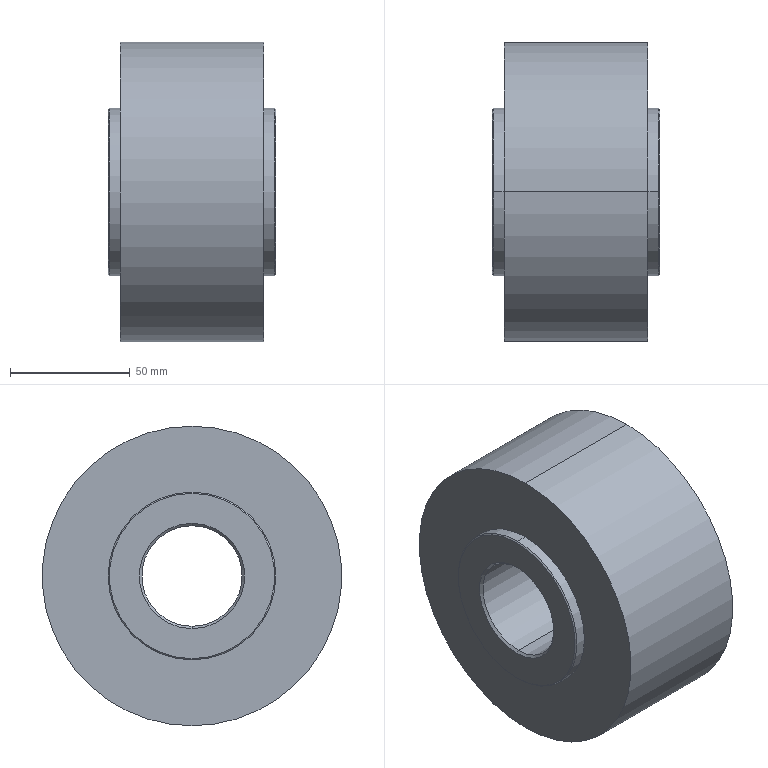Part | SolidWorks | features BaseBody 1 | 1 solid | 28 faces | box 70 x 125 x 125 mm | volume 635681 mm3 | cylinder 12 | cone 10 | plane 6 | commonest cylinder face diameters 70 x4 42 x2 52 x2 62 x2 125 x2
STEP:
#1=CARTESIAN_POINT('',(-30.,0.,-62.5));
#2=VERTEX_POINT('',#1);
#3=CARTESIAN_POINT('',(-30.,0.,62.5));
#4=VERTEX_POINT('',#3);
#5=CARTESIAN_POINT('',(-30.,0.,0.));
#6=DIRECTION('',(1.,0.,0.));
#7=DIRECTION('',(0.,0.,-1.));
#8=AXIS2_PLACEMENT_3D('',#5,#6,#7);
#9=CIRCLE('',#8,62.5);
#10=EDGE_CURVE('',#2,#4,#9,.T.);
#11=ORIENTED_EDGE('',*,*,#10,.T.);
#12=CARTESIAN_POINT('',(30.,0.,62.5));
#13=VERTEX_POINT('',#12);
#14=CARTESIAN_POINT('',(-38.5,0.,62.5));
#15=DIRECTION('',(1.,0.,0.));
#16=VECTOR('',#15,1000.);
#17=LINE('',#14,#16);
#18=EDGE_CURVE('',#4,#13,#17,.T.);
#19=ORIENTED_EDGE('',*,*,#18,.T.);
#20=CARTESIAN_POINT('',(30.,0.,-62.5));
#21=VERTEX_POINT('',#20);
#22=CARTESIAN_POINT('',(30.,0.,0.));
#23=DIRECTION('',(-1.,0.,0.));
#24=DIRECTION('',(0.,0.,-1.));
#25=AXIS2_PLACEMENT_3D('',#22,#23,#24);
#26=CIRCLE('',#25,62.5);
#27=EDGE_CURVE('',#13,#21,#26,.T.);
#28=ORIENTED_EDGE('',*,*,#27,.T.);
#29=CARTESIAN_POINT('',(-38.5,0.,-62.5));
#30=DIRECTION('',(1.,0.,0.));
#31=VECTOR('',#30,1000.);
#32=LINE('',#29,#31);
#33=EDGE_CURVE('',#2,#21,#32,.T.);
#34=ORIENTED_EDGE('',*,*,#33,.F.);
#35=EDGE_LOOP('',(#11,#19,#28,#34));
#36=FACE_OUTER_BOUND('',#35,.T.);
#37=CARTESIAN_POINT('',(-38.5,0.,0.));
#38=DIRECTION('',(1.,0.,0.));
#39=DIRECTION('',(0.,0.,-1.));
#40=AXIS2_PLACEMENT_3D('',#37,#38,#39);
#41=CYLINDRICAL_SURFACE('',#40,62.5);
#42=ADVANCED_FACE('',(#36),#41,.T.);
#43=CARTESIAN_POINT('',(30.,0.,35.));
#44=VERTEX_POINT('',#43);
#45=CARTESIAN_POINT('',(30.,0.,-35.));
#46=VERTEX_POINT('',#45);
#47=CARTESIAN_POINT('',(30.,0.,0.));
#48=DIRECTION('',(-1.,0.,0.));
#49=DIRECTION('',(0.,0.,-1.));
#50=AXIS2_PLACEMENT_3D('',#47,#48,#49);
#51=CIRCLE('',#50,35.);
#52=EDGE_CURVE('',#44,#46,#51,.T.);
#53=ORIENTED_EDGE('',*,*,#52,.F.);
#54=CARTESIAN_POINT('',(34.5,0.,35.));
#55=VERTEX_POINT('',#54);
#56=CARTESIAN_POINT('',(-38.5,0.,35.));
#57=DIRECTION('',(1.,0.,0.));
#58=VECTOR('',#57,1000.);
#59=LINE('',#56,#58);
#60=EDGE_CURVE('',#44,#55,#59,.T.);
#61=ORIENTED_EDGE('',*,*,#60,.T.);
#62=CARTESIAN_POINT('',(34.5,0.,-35.));
#63=VERTEX_POINT('',#62);
#64=CARTESIAN_POINT('',(34.5,0.,0.));
#65=DIRECTION('',(-1.,0.,0.));
#66=DIRECTION('',(0.,0.,-1.));
#67=AXIS2_PLACEMENT_3D('',#64,#65,#66);
#68=CIRCLE('',#67,35.);
#69=EDGE_CURVE('',#55,#63,#68,.T.);
#70=ORIENTED_EDGE('',*,*,#69,.T.);
#71=CARTESIAN_POINT('',(-38.5,0.,-35.));
#72=DIRECTION('',(1.,0.,0.));
#73=VECTOR('',#72,1000.);
#74=LINE('',#71,#73);
#75=EDGE_CURVE('',#46,#63,#74,.T.);
#76=ORIENTED_EDGE('',*,*,#75,.F.);
#77=EDGE_LOOP('',(#53,#61,#70,#76));
#78=FACE_OUTER_BOUND('',#77,.T.);
#79=CARTESIAN_POINT('',(-38.5,0.,0.));
#80=DIRECTION('',(1.,0.,0.));
#81=DIRECTION('',(0.,0.,-1.));
#82=AXIS2_PLACEMENT_3D('',#79,#80,#81);
#83=CYLINDRICAL_SURFACE('',#82,35.);
#84=ADVANCED_FACE('',(#78),#83,.T.);
#85=CARTESIAN_POINT('',(-34.5,0.,-35.));
#86=VERTEX_POINT('',#85);
#87=CARTESIAN_POINT('',(-34.5,0.,35.));
#88=VERTEX_POINT('',#87);
#89=CARTESIAN_POINT('',(-34.5,0.,0.));
#90=DIRECTION('',(1.,0.,0.));
#91=DIRECTION('',(0.,0.,-1.));
#92=AXIS2_PLACEMENT_3D('',#89,#90,#91);
#93=CIRCLE('',#92,35.);
#94=EDGE_CURVE('',#86,#88,#93,.T.);
#95=ORIENTED_EDGE('',*,*,#94,.T.);
#96=CARTESIAN_POINT('',(-30.,0.,35.));
#97=VERTEX_POINT('',#96);
#98=CARTESIAN_POINT('',(-38.5,0.,35.));
#99=DIRECTION('',(1.,0.,0.));
#100=VECTOR('',#99,1000.);
#101=LINE('',#98,#100);
#102=EDGE_CURVE('',#88,#97,#101,.T.);
#103=ORIENTED_EDGE('',*,*,#102,.T.);
#104=CARTESIAN_POINT('',(-30.,0.,-35.));
#105=VERTEX_POINT('',#104);
#106=CARTESIAN_POINT('',(-30.,0.,0.));
#107=DIRECTION('',(-1.,0.,0.));
#108=DIRECTION('',(0.,0.,-1.));
#109=AXIS2_PLACEMENT_3D('',#106,#107,#108);
#110=CIRCLE('',#109,35.);
#111=EDGE_CURVE('',#97,#105,#110,.T.);
#112=ORIENTED_EDGE('',*,*,#111,.T.);
#113=CARTESIAN_POINT('',(-38.5,0.,-35.));
#114=DIRECTION('',(1.,0.,0.));
#115=VECTOR('',#114,1000.);
#116=LINE('',#113,#115);
#117=EDGE_CURVE('',#86,#105,#116,.T.);
#118=ORIENTED_EDGE('',*,*,#117,.F.);
#119=EDGE_LOOP('',(#95,#103,#112,#118));
#120=FACE_OUTER_BOUND('',#119,.T.);
#121=CARTESIAN_POINT('',(-38.5,0.,0.));
#122=DIRECTION('',(1.,0.,0.));
#123=DIRECTION('',(0.,0.,-1.));
#124=AXIS2_PLACEMENT_3D('',#121,#122,#123);
#125=CYLINDRICAL_SURFACE('',#124,35.);
#126=ADVANCED_FACE('',(#120),#125,.T.);
#127=CARTESIAN_POINT('',(35.,0.,34.5));
#128=VERTEX_POINT('',#127);
#129=CARTESIAN_POINT('',(35.,0.,-34.5));
#130=VERTEX_POINT('',#129);
#131=CARTESIAN_POINT('',(35.,0.,0.));
#132=DIRECTION('',(-1.,0.,0.));
#133=DIRECTION('',(0.,0.,1.));
#134=AXIS2_PLACEMENT_3D('',#131,#132,#133);
#135=CIRCLE('',#134,34.5);
#136=EDGE_CURVE('',#128,#130,#135,.T.);
#137=ORIENTED_EDGE('',*,*,#136,.T.);
#138=CARTESIAN_POINT('',(34.5,0.,-35.));
#139=DIRECTION('',(-0.7071,0.,-0.7071));
#140=VECTOR('',#139,1000.);
#141=LINE('',#138,#140);
#142=EDGE_CURVE('',#130,#63,#141,.T.);
#143=ORIENTED_EDGE('',*,*,#142,.T.);
#144=ORIENTED_EDGE('',*,*,#69,.F.);
#145=CARTESIAN_POINT('',(34.5,0.,35.));
#146=DIRECTION('',(-0.7071,0.,0.7071));
#147=VECTOR('',#146,1000.);
#148=LINE('',#145,#147);
#149=EDGE_CURVE('',#128,#55,#148,.T.);
#150=ORIENTED_EDGE('',*,*,#149,.F.);
#151=EDGE_LOOP('',(#137,#143,#144,#150));
#152=FACE_OUTER_BOUND('',#151,.T.);
#153=CARTESIAN_POINT('',(34.5,0.,0.));
#154=DIRECTION('',(-1.,0.,0.));
#155=DIRECTION('',(0.,0.,1.));
#156=AXIS2_PLACEMENT_3D('',#153,#154,#155);
#157=CONICAL_SURFACE('',#156,35.,0.7854);
#158=ADVANCED_FACE('',(#152),#157,.T.);
#159=CARTESIAN_POINT('',(-35.,0.,-34.5));
#160=VERTEX_POINT('',#159);
#161=CARTESIAN_POINT('',(-35.,0.,34.5));
#162=VERTEX_POINT('',#161);
#163=CARTESIAN_POINT('',(-35.,0.,0.));
#164=DIRECTION('',(1.,0.,0.));
#165=DIRECTION('',(0.,0.,-1.));
#166=AXIS2_PLACEMENT_3D('',#163,#164,#165);
#167=CIRCLE('',#166,34.5);
#168=EDGE_CURVE('',#160,#162,#167,.T.);
#169=ORIENTED_EDGE('',*,*,#168,.T.);
#170=CARTESIAN_POINT('',(-34.5,0.,35.));
#171=DIRECTION('',(0.7071,0.,0.7071));
#172=VECTOR('',#171,1000.);
#173=LINE('',#170,#172);
#174=EDGE_CURVE('',#162,#88,#173,.T.);
#175=ORIENTED_EDGE('',*,*,#174,.T.);
#176=ORIENTED_EDGE('',*,*,#94,.F.);
#177=CARTESIAN_POINT('',(-34.5,0.,-35.));
#178=DIRECTION('',(0.7071,0.,-0.7071));
#179=VECTOR('',#178,1000.);
#180=LINE('',#177,#179);
#181=EDGE_CURVE('',#160,#86,#180,.T.);
#182=ORIENTED_EDGE('',*,*,#181,.F.);
#183=EDGE_LOOP('',(#169,#175,#176,#182));
#184=FACE_OUTER_BOUND('',#183,.T.);
#185=CARTESIAN_POINT('',(-34.5,0.,0.));
#186=DIRECTION('',(1.,0.,0.));
#187=DIRECTION('',(0.,0.,-1.));
#188=AXIS2_PLACEMENT_3D('',#185,#186,#187);
#189=CONICAL_SURFACE('',#188,35.,0.7854);
#190=ADVANCED_FACE('',(#184),#189,.T.);
#191=CARTESIAN_POINT('',(34.,0.,31.));
#192=VERTEX_POINT('',#191);
#193=CARTESIAN_POINT('',(34.,0.,-31.));
#194=VERTEX_POINT('',#193);
#195=CARTESIAN_POINT('',(34.,0.,0.));
#196=DIRECTION('',(1.,0.,0.));
#197=DIRECTION('',(0.,0.,-1.));
#198=AXIS2_PLACEMENT_3D('',#195,#196,#197);
#199=CIRCLE('',#198,31.);
#200=EDGE_CURVE('',#192,#194,#199,.T.);
#201=ORIENTED_EDGE('',*,*,#200,.F.);
#202=CARTESIAN_POINT('',(35.,0.,32.));
#203=VERTEX_POINT('',#202);
#204=CARTESIAN_POINT('',(35.,0.,32.));
#205=DIRECTION('',(0.7071,0.,0.7071));
#206=VECTOR('',#205,1000.);
#207=LINE('',#204,#206);
#208=EDGE_CURVE('',#192,#203,#207,.T.);
#209=ORIENTED_EDGE('',*,*,#208,.T.);
#210=CARTESIAN_POINT('',(35.,0.,-32.));
#211=VERTEX_POINT('',#210);
#212=CARTESIAN_POINT('',(35.,0.,0.));
#213=DIRECTION('',(-1.,0.,0.));
#214=DIRECTION('',(0.,0.,-1.));
#215=AXIS2_PLACEMENT_3D('',#212,#213,#214);
#216=CIRCLE('',#215,32.);
#217=EDGE_CURVE('',#211,#203,#216,.T.);
#218=ORIENTED_EDGE('',*,*,#217,.F.);
#219=CARTESIAN_POINT('',(35.,0.,-32.));
#220=DIRECTION('',(0.7071,0.,-0.7071));
#221=VECTOR('',#220,1000.);
#222=LINE('',#219,#221);
#223=EDGE_CURVE('',#194,#211,#222,.T.);
#224=ORIENTED_EDGE('',*,*,#223,.F.);
#225=EDGE_LOOP('',(#201,#209,#218,#224));
#226=FACE_OUTER_BOUND('',#225,.T.);
#227=CARTESIAN_POINT('',(35.,0.,0.));
#228=DIRECTION('',(1.,0.,0.));
#229=DIRECTION('',(0.,0.,-1.));
#230=AXIS2_PLACEMENT_3D('',#227,#228,#229);
#231=CONICAL_SURFACE('',#230,32.,0.7854);
#232=ADVANCED_FACE('',(#226),#231,.F.);
#233=CARTESIAN_POINT('',(-34.,0.,-21.));
#234=VERTEX_POINT('',#233);
#235=CARTESIAN_POINT('',(-34.,0.,21.));
#236=VERTEX_POINT('',#235);
#237=CARTESIAN_POINT('',(-34.,0.,0.));
#238=DIRECTION('',(-1.,0.,0.));
#239=DIRECTION('',(0.,0.,-1.));
#240=AXIS2_PLACEMENT_3D('',#237,#238,#239);
#241=CIRCLE('',#240,21.);
#242=EDGE_CURVE('',#234,#236,#241,.T.);
#243=ORIENTED_EDGE('',*,*,#242,.F.);
#244=CARTESIAN_POINT('',(-35.,0.,-22.));
#245=VERTEX_POINT('',#244);
#246=CARTESIAN_POINT('',(-35.,0.,-22.));
#247=DIRECTION('',(-0.7071,0.,-0.7071));
#248=VECTOR('',#247,1000.);
#249=LINE('',#246,#248);
#250=EDGE_CURVE('',#234,#245,#249,.T.);
#251=ORIENTED_EDGE('',*,*,#250,.T.);
#252=CARTESIAN_POINT('',(-35.,0.,22.));
#253=VERTEX_POINT('',#252);
#254=CARTESIAN_POINT('',(-35.,0.,0.));
#255=DIRECTION('',(-1.,0.,0.));
#256=DIRECTION('',(0.,0.,1.));
#257=AXIS2_PLACEMENT_3D('',#254,#255,#256);
#258=CIRCLE('',#257,22.);
#259=EDGE_CURVE('',#245,#253,#258,.T.);
#260=ORIENTED_EDGE('',*,*,#259,.T.);
#261=CARTESIAN_POINT('',(-35.,0.,22.));
#262=DIRECTION('',(-0.7071,0.,0.7071));
#263=VECTOR('',#262,1000.);
#264=LINE('',#261,#263);
#265=EDGE_CURVE('',#236,#253,#264,.T.);
#266=ORIENTED_EDGE('',*,*,#265,.F.);
#267=EDGE_LOOP('',(#243,#251,#260,#266));
#268=FACE_OUTER_BOUND('',#267,.T.);
#269=CARTESIAN_POINT('',(-35.,0.,0.));
#270=DIRECTION('',(-1.,0.,0.));
#271=DIRECTION('',(0.,0.,1.));
#272=AXIS2_PLACEMENT_3D('',#269,#270,#271);
#273=CONICAL_SURFACE('',#272,22.,0.7854);
#274=ADVANCED_FACE('',(#268),#273,.F.);
#275=CARTESIAN_POINT('',(13.,0.,31.));
#276=VERTEX_POINT('',#275);
#277=CARTESIAN_POINT('',(13.,0.,-31.));
#278=VERTEX_POINT('',#277);
#279=CARTESIAN_POINT('',(13.,0.,0.));
#280=DIRECTION('',(1.,0.,0.));
#281=DIRECTION('',(0.,0.,-1.));
#282=AXIS2_PLACEMENT_3D('',#279,#280,#281);
#283=CIRCLE('',#282,31.);
#284=EDGE_CURVE('',#276,#278,#283,.T.);
#285=ORIENTED_EDGE('',*,*,#284,.F.);
#286=CARTESIAN_POINT('',(-38.5,0.,31.));
#287=DIRECTION('',(1.,0.,0.));
#288=VECTOR('',#287,1000.);
#289=LINE('',#286,#288);
#290=EDGE_CURVE('',#276,#192,#289,.T.);
#291=ORIENTED_EDGE('',*,*,#290,.T.);
#292=ORIENTED_EDGE('',*,*,#200,.T.);
#293=CARTESIAN_POINT('',(-38.5,0.,-31.));
#294=DIRECTION('',(1.,0.,0.));
#295=VECTOR('',#294,1000.);
#296=LINE('',#293,#295);
#297=EDGE_CURVE('',#278,#194,#296,.T.);
#298=ORIENTED_EDGE('',*,*,#297,.F.);
#299=EDGE_LOOP('',(#285,#291,#292,#298));
#300=FACE_OUTER_BOUND('',#299,.T.);
#301=CARTESIAN_POINT('',(-38.5,0.,0.));
#302=DIRECTION('',(1.,0.,0.));
#303=DIRECTION('',(0.,0.,-1.));
#304=AXIS2_PLACEMENT_3D('',#301,#302,#303);
#305=CYLINDRICAL_SURFACE('',#304,31.);
#306=ADVANCED_FACE('',(#300),#305,.F.);
#307=ORIENTED_EDGE('',*,*,#242,.T.);
#308=CARTESIAN_POINT('',(4.,0.,21.));
#309=VERTEX_POINT('',#308);
#310=CARTESIAN_POINT('',(-38.5,0.,21.));
#311=DIRECTION('',(1.,0.,0.));
#312=VECTOR('',#311,1000.);
#313=LINE('',#310,#312);
#314=EDGE_CURVE('',#236,#309,#313,.T.);
#315=ORIENTED_EDGE('',*,*,#314,.T.);
#316=CARTESIAN_POINT('',(4.,0.,-21.));
#317=VERTEX_POINT('',#316);
#318=CARTESIAN_POINT('',(4.,0.,0.));
#319=DIRECTION('',(-1.,0.,0.));
#320=DIRECTION('',(0.,0.,-1.));
#321=AXIS2_PLACEMENT_3D('',#318,#319,#320);
#322=CIRCLE('',#321,21.);
#323=EDGE_CURVE('',#317,#309,#322,.T.);
#324=ORIENTED_EDGE('',*,*,#323,.F.);
#325=CARTESIAN_POINT('',(-38.5,0.,-21.));
#326=DIRECTION('',(1.,0.,0.));
#327=VECTOR('',#326,1000.);
#328=LINE('',#325,#327);
#329=EDGE_CURVE('',#234,#317,#328,.T.);
#330=ORIENTED_EDGE('',*,*,#329,.F.);
#331=EDGE_LOOP('',(#307,#315,#324,#330));
#332=FACE_OUTER_BOUND('',#331,.T.);
#333=CARTESIAN_POINT('',(-38.5,0.,0.));
#334=DIRECTION('',(1.,0.,0.));
#335=DIRECTION('',(0.,0.,-1.));
#336=AXIS2_PLACEMENT_3D('',#333,#334,#335);
#337=CYLINDRICAL_SURFACE('',#336,21.);
#338=ADVANCED_FACE('',(#332),#337,.F.);
#339=ORIENTED_EDGE('',*,*,#323,.T.);
#340=CARTESIAN_POINT('',(5.,0.,22.));
#341=VERTEX_POINT('',#340);
#342=CARTESIAN_POINT('',(5.,0.,22.));
#343=DIRECTION('',(0.7071,0.,0.7071));
#344=VECTOR('',#343,1000.);
#345=LINE('',#342,#344);
#346=EDGE_CURVE('',#309,#341,#345,.T.);
#347=ORIENTED_EDGE('',*,*,#346,.T.);
#348=CARTESIAN_POINT('',(5.,0.,-22.));
#349=VERTEX_POINT('',#348);
#350=CARTESIAN_POINT('',(5.,0.,0.));
#351=DIRECTION('',(-1.,0.,0.));
#352=DIRECTION('',(0.,0.,-1.));
#353=AXIS2_PLACEMENT_3D('',#350,#351,#352);
#354=CIRCLE('',#353,22.);
#355=EDGE_CURVE('',#349,#341,#354,.T.);
#356=ORIENTED_EDGE('',*,*,#355,.F.);
#357=CARTESIAN_POINT('',(5.,0.,-22.));
#358=DIRECTION('',(0.7071,0.,-0.7071));
#359=VECTOR('',#358,1000.);
#360=LINE('',#357,#359);
#361=EDGE_CURVE('',#317,#349,#360,.T.);
#362=ORIENTED_EDGE('',*,*,#361,.F.);
#363=EDGE_LOOP('',(#339,#347,#356,#362));
#364=FACE_OUTER_BOUND('',#363,.T.);
#365=CARTESIAN_POINT('',(5.,0.,0.));
#366=DIRECTION('',(1.,0.,0.));
#367=DIRECTION('',(0.,0.,-1.));
#368=AXIS2_PLACEMENT_3D('',#365,#366,#367);
#369=CONICAL_SURFACE('',#368,22.,0.7854);
#370=ADVANCED_FACE('',(#364),#369,.F.);
#371=CARTESIAN_POINT('',(5.,0.,26.));
#372=VERTEX_POINT('',#371);
#373=CARTESIAN_POINT('',(5.,0.,-26.));
#374=VERTEX_POINT('',#373);
#375=CARTESIAN_POINT('',(5.,0.,0.));
#376=DIRECTION('',(1.,0.,0.));
#377=DIRECTION('',(0.,0.,-1.));
#378=AXIS2_PLACEMENT_3D('',#375,#376,#377);
#379=CIRCLE('',#378,26.);
#380=EDGE_CURVE('',#372,#374,#379,.T.);
#381=ORIENTED_EDGE('',*,*,#380,.F.);
#382=CARTESIAN_POINT('',(13.,0.,26.));
#383=VERTEX_POINT('',#382);
#384=CARTESIAN_POINT('',(-38.5,0.,26.));
#385=DIRECTION('',(1.,0.,0.));
#386=VECTOR('',#385,1000.);
#387=LINE('',#384,#386);
#388=EDGE_CURVE('',#372,#383,#387,.T.);
#389=ORIENTED_EDGE('',*,*,#388,.T.);
#390=CARTESIAN_POINT('',(13.,0.,-26.));
#391=VERTEX_POINT('',#390);
#392=CARTESIAN_POINT('',(13.,0.,0.));
#393=DIRECTION('',(-1.,0.,0.));
#394=DIRECTION('',(0.,0.,-1.));
#395=AXIS2_PLACEMENT_3D('',#392,#393,#394);
#396=CIRCLE('',#395,26.);
#397=EDGE_CURVE('',#391,#383,#396,.T.);
#398=ORIENTED_EDGE('',*,*,#397,.F.);
#399=CARTESIAN_POINT('',(-38.5,0.,-26.));
#400=DIRECTION('',(1.,0.,0.));
#401=VECTOR('',#400,1000.);
#402=LINE('',#399,#401);
#403=EDGE_CURVE('',#374,#391,#402,.T.);
#404=ORIENTED_EDGE('',*,*,#403,.F.);
#405=EDGE_LOOP('',(#381,#389,#398,#404));
#406=FACE_OUTER_BOUND('',#405,.T.);
#407=CARTESIAN_POINT('',(-38.5,0.,0.));
#408=DIRECTION('',(1.,0.,0.));
#409=DIRECTION('',(0.,0.,-1.));
#410=AXIS2_PLACEMENT_3D('',#407,#408,#409);
#411=CYLINDRICAL_SURFACE('',#410,26.);
#412=ADVANCED_FACE('',(#406),#411,.F.);
#413=ORIENTED_EDGE('',*,*,#18,.F.);
#414=CARTESIAN_POINT('',(-30.,0.,0.));
#415=DIRECTION('',(1.,0.,0.));
#416=DIRECTION('',(0.,0.,-1.));
#417=AXIS2_PLACEMENT_3D('',#414,#415,#416);
#418=CIRCLE('',#417,62.5);
#419=EDGE_CURVE('',#4,#2,#418,.T.);
#420=ORIENTED_EDGE('',*,*,#419,.T.);
#421=ORIENTED_EDGE('',*,*,#33,.T.);
#422=CARTESIAN_POINT('',(30.,0.,0.));
#423=DIRECTION('',(-1.,0.,0.));
#424=DIRECTION('',(0.,0.,-1.));
#425=AXIS2_PLACEMENT_3D('',#422,#423,#424);
#426=CIRCLE('',#425,62.5);
#427=EDGE_CURVE('',#21,#13,#426,.T.);
#428=ORIENTED_EDGE('',*,*,#427,.T.);
#429=EDGE_LOOP('',(#413,#420,#421,#428));
#430=FACE_OUTER_BOUND('',#429,.T.);
#431=CARTESIAN_POINT('',(-38.5,0.,0.));
#432=DIRECTION('',(1.,0.,0.));
#433=DIRECTION('',(0.,0.,-1.));
#434=AXIS2_PLACEMENT_3D('',#431,#432,#433);
#435=CYLINDRICAL_SURFACE('',#434,62.5);
#436=ADVANCED_FACE('',(#430),#435,.T.);
#437=CARTESIAN_POINT('',(30.,0.,0.));
#438=DIRECTION('',(-1.,0.,0.));
#439=DIRECTION('',(0.,0.,-1.));
#440=AXIS2_PLACEMENT_3D('',#437,#438,#439);
#441=CIRCLE('',#440,35.);
#442=EDGE_CURVE('',#46,#44,#441,.T.);
#443=ORIENTED_EDGE('',*,*,#442,.T.);
#444=ORIENTED_EDGE('',*,*,#52,.T.);
#445=EDGE_LOOP('',(#443,#444));
#446=FACE_BOUND('',#445,.T.);
#447=ORIENTED_EDGE('',*,*,#427,.F.);
#448=ORIENTED_EDGE('',*,*,#27,.F.);
#449=EDGE_LOOP('',(#447,#448));
#450=FACE_OUTER_BOUND('',#449,.T.);
#451=CARTESIAN_POINT('',(30.,0.,0.));
#452=DIRECTION('',(1.,0.,0.));
#453=DIRECTION('',(0.,0.,-1.));
#454=AXIS2_PLACEMENT_3D('',#451,#452,#453);
#455=PLANE('',#454);
#456=ADVANCED_FACE('',(#446,#450),#455,.T.);
#457=CARTESIAN_POINT('',(-30.,0.,0.));
#458=DIRECTION('',(-1.,0.,0.));
#459=DIRECTION('',(0.,0.,-1.));
#460=AXIS2_PLACEMENT_3D('',#457,#458,#459);
#461=CIRCLE('',#460,35.);
#462=EDGE_CURVE('',#105,#97,#461,.T.);
#463=ORIENTED_EDGE('',*,*,#462,.F.);
#464=ORIENTED_EDGE('',*,*,#111,.F.);
#465=EDGE_LOOP('',(#463,#464));
#466=FACE_BOUND('',#465,.T.);
#467=ORIENTED_EDGE('',*,*,#10,.F.);
#468=ORIENTED_EDGE('',*,*,#419,.F.);
#469=EDGE_LOOP('',(#467,#468));
#470=FACE_OUTER_BOUND('',#469,.T.);
#471=CARTESIAN_POINT('',(-30.,0.,0.));
#472=DIRECTION('',(1.,0.,0.));
#473=DIRECTION('',(0.,0.,-1.));
#474=AXIS2_PLACEMENT_3D('',#471,#472,#473);
#475=PLANE('',#474);
#476=ADVANCED_FACE('',(#466,#470),#475,.F.);
#477=ORIENTED_EDGE('',*,*,#60,.F.);
#478=ORIENTED_EDGE('',*,*,#442,.F.);
#479=ORIENTED_EDGE('',*,*,#75,.T.);
#480=CARTESIAN_POINT('',(34.5,0.,0.));
#481=DIRECTION('',(-1.,0.,0.));
#482=DIRECTION('',(0.,0.,-1.));
#483=AXIS2_PLACEMENT_3D('',#480,#481,#482);
#484=CIRCLE('',#483,35.);
#485=EDGE_CURVE('',#63,#55,#484,.T.);
#486=ORIENTED_EDGE('',*,*,#485,.T.);
#487=EDGE_LOOP('',(#477,#478,#479,#486));
#488=FACE_OUTER_BOUND('',#487,.T.);
#489=CARTESIAN_POINT('',(-38.5,0.,0.));
#490=DIRECTION('',(1.,0.,0.));
#491=DIRECTION('',(0.,0.,-1.));
#492=AXIS2_PLACEMENT_3D('',#489,#490,#491);
#493=CYLINDRICAL_SURFACE('',#492,35.);
#494=ADVANCED_FACE('',(#488),#493,.T.);
#495=ORIENTED_EDGE('',*,*,#102,.F.);
#496=CARTESIAN_POINT('',(-34.5,0.,0.));
#497=DIRECTION('',(1.,0.,0.));
#498=DIRECTION('',(0.,0.,-1.));
#499=AXIS2_PLACEMENT_3D('',#496,#497,#498);
#500=CIRCLE('',#499,35.);
#501=EDGE_CURVE('',#88,#86,#500,.T.);
#502=ORIENTED_EDGE('',*,*,#501,.T.);
#503=ORIENTED_EDGE('',*,*,#117,.T.);
#504=ORIENTED_EDGE('',*,*,#462,.T.);
#505=EDGE_LOOP('',(#495,#502,#503,#504));
#506=FACE_OUTER_BOUND('',#505,.T.);
#507=CARTESIAN_POINT('',(-38.5,0.,0.));
#508=DIRECTION('',(1.,0.,0.));
#509=DIRECTION('',(0.,0.,-1.));
#510=AXIS2_PLACEMENT_3D('',#507,#508,#509);
#511=CYLINDRICAL_SURFACE('',#510,35.);
#512=ADVANCED_FACE('',(#506),#511,.T.);
#513=ORIENTED_EDGE('',*,*,#142,.F.);
#514=CARTESIAN_POINT('',(35.,0.,0.));
#515=DIRECTION('',(-1.,0.,0.));
#516=DIRECTION('',(0.,0.,1.));
#517=AXIS2_PLACEMENT_3D('',#514,#515,#516);
#518=CIRCLE('',#517,34.5);
#519=EDGE_CURVE('',#130,#128,#518,.T.);
#520=ORIENTED_EDGE('',*,*,#519,.T.);
#521=ORIENTED_EDGE('',*,*,#149,.T.);
#522=ORIENTED_EDGE('',*,*,#485,.F.);
#523=EDGE_LOOP('',(#513,#520,#521,#522));
#524=FACE_OUTER_BOUND('',#523,.T.);
#525=CARTESIAN_POINT('',(34.5,0.,0.));
#526=DIRECTION('',(-1.,0.,0.));
#527=DIRECTION('',(0.,0.,1.));
#528=AXIS2_PLACEMENT_3D('',#525,#526,#527);
#529=CONICAL_SURFACE('',#528,35.,0.7854);
#530=ADVANCED_FACE('',(#524),#529,.T.);
#531=ORIENTED_EDGE('',*,*,#174,.F.);
#532=CARTESIAN_POINT('',(-35.,0.,0.));
#533=DIRECTION('',(1.,0.,0.));
#534=DIRECTION('',(0.,0.,-1.));
#535=AXIS2_PLACEMENT_3D('',#532,#533,#534);
#536=CIRCLE('',#535,34.5);
#537=EDGE_CURVE('',#162,#160,#536,.T.);
#538=ORIENTED_EDGE('',*,*,#537,.T.);
#539=ORIENTED_EDGE('',*,*,#181,.T.);
#540=ORIENTED_EDGE('',*,*,#501,.F.);
#541=EDGE_LOOP('',(#531,#538,#539,#540));
#542=FACE_OUTER_BOUND('',#541,.T.);
#543=CARTESIAN_POINT('',(-34.5,0.,0.));
#544=DIRECTION('',(1.,0.,0.));
#545=DIRECTION('',(0.,0.,-1.));
#546=AXIS2_PLACEMENT_3D('',#543,#544,#545);
#547=CONICAL_SURFACE('',#546,35.,0.7854);
#548=ADVANCED_FACE('',(#542),#547,.T.);
#549=ORIENTED_EDGE('',*,*,#217,.T.);
#550=CARTESIAN_POINT('',(35.,0.,0.));
#551=DIRECTION('',(-1.,0.,0.));
#552=DIRECTION('',(0.,0.,-1.));
#553=AXIS2_PLACEMENT_3D('',#550,#551,#552);
#554=CIRCLE('',#553,32.);
#555=EDGE_CURVE('',#203,#211,#554,.T.);
#556=ORIENTED_EDGE('',*,*,#555,.T.);
#557=EDGE_LOOP('',(#549,#556));
#558=FACE_BOUND('',#557,.T.);
#559=ORIENTED_EDGE('',*,*,#136,.F.);
#560=ORIENTED_EDGE('',*,*,#519,.F.);
#561=EDGE_LOOP('',(#559,#560));
#562=FACE_OUTER_BOUND('',#561,.T.);
#563=CARTESIAN_POINT('',(35.,0.,0.));
#564=DIRECTION('',(1.,0.,0.));
#565=DIRECTION('',(0.,0.,-1.));
#566=AXIS2_PLACEMENT_3D('',#563,#564,#565);
#567=PLANE('',#566);
#568=ADVANCED_FACE('',(#558,#562),#567,.T.);
#569=CARTESIAN_POINT('',(-35.,0.,0.));
#570=DIRECTION('',(-1.,0.,0.));
#571=DIRECTION('',(0.,0.,1.));
#572=AXIS2_PLACEMENT_3D('',#569,#570,#571);
#573=CIRCLE('',#572,22.);
#574=EDGE_CURVE('',#253,#245,#573,.T.);
#575=ORIENTED_EDGE('',*,*,#574,.F.);
#576=ORIENTED_EDGE('',*,*,#259,.F.);
#577=EDGE_LOOP('',(#575,#576));
#578=FACE_BOUND('',#577,.T.);
#579=ORIENTED_EDGE('',*,*,#168,.F.);
#580=ORIENTED_EDGE('',*,*,#537,.F.);
#581=EDGE_LOOP('',(#579,#580));
#582=FACE_OUTER_BOUND('',#581,.T.);
#583=CARTESIAN_POINT('',(-35.,0.,0.));
#584=DIRECTION('',(1.,0.,0.));
#585=DIRECTION('',(0.,0.,-1.));
#586=AXIS2_PLACEMENT_3D('',#583,#584,#585);
#587=PLANE('',#586);
#588=ADVANCED_FACE('',(#578,#582),#587,.F.);
#589=ORIENTED_EDGE('',*,*,#208,.F.);
#590=CARTESIAN_POINT('',(34.,0.,0.));
#591=DIRECTION('',(1.,0.,0.));
#592=DIRECTION('',(0.,0.,-1.));
#593=AXIS2_PLACEMENT_3D('',#590,#591,#592);
#594=CIRCLE('',#593,31.);
#595=EDGE_CURVE('',#194,#192,#594,.T.);
#596=ORIENTED_EDGE('',*,*,#595,.F.);
#597=ORIENTED_EDGE('',*,*,#223,.T.);
#598=ORIENTED_EDGE('',*,*,#555,.F.);
#599=EDGE_LOOP('',(#589,#596,#597,#598));
#600=FACE_OUTER_BOUND('',#599,.T.);
#601=CARTESIAN_POINT('',(35.,0.,0.));
#602=DIRECTION('',(1.,0.,0.));
#603=DIRECTION('',(0.,0.,-1.));
#604=AXIS2_PLACEMENT_3D('',#601,#602,#603);
#605=CONICAL_SURFACE('',#604,32.,0.7854);
#606=ADVANCED_FACE('',(#600),#605,.F.);
#607=ORIENTED_EDGE('',*,*,#250,.F.);
#608=CARTESIAN_POINT('',(-34.,0.,0.));
#609=DIRECTION('',(-1.,0.,0.));
#610=DIRECTION('',(0.,0.,-1.));
#611=AXIS2_PLACEMENT_3D('',#608,#609,#610);
#612=CIRCLE('',#611,21.);
#613=EDGE_CURVE('',#236,#234,#612,.T.);
#614=ORIENTED_EDGE('',*,*,#613,.F.);
#615=ORIENTED_EDGE('',*,*,#265,.T.);
#616=ORIENTED_EDGE('',*,*,#574,.T.);
#617=EDGE_LOOP('',(#607,#614,#615,#616));
#618=FACE_OUTER_BOUND('',#617,.T.);
#619=CARTESIAN_POINT('',(-35.,0.,0.));
#620=DIRECTION('',(-1.,0.,0.));
#621=DIRECTION('',(0.,0.,1.));
#622=AXIS2_PLACEMENT_3D('',#619,#620,#621);
#623=CONICAL_SURFACE('',#622,22.,0.7854);
#624=ADVANCED_FACE('',(#618),#623,.F.);
#625=ORIENTED_EDGE('',*,*,#290,.F.);
#626=CARTESIAN_POINT('',(13.,0.,0.));
#627=DIRECTION('',(1.,0.,0.));
#628=DIRECTION('',(0.,0.,-1.));
#629=AXIS2_PLACEMENT_3D('',#626,#627,#628);
#630=CIRCLE('',#629,31.);
#631=EDGE_CURVE('',#278,#276,#630,.T.);
#632=ORIENTED_EDGE('',*,*,#631,.F.);
#633=ORIENTED_EDGE('',*,*,#297,.T.);
#634=ORIENTED_EDGE('',*,*,#595,.T.);
#635=EDGE_LOOP('',(#625,#632,#633,#634));
#636=FACE_OUTER_BOUND('',#635,.T.);
#637=CARTESIAN_POINT('',(-38.5,0.,0.));
#638=DIRECTION('',(1.,0.,0.));
#639=DIRECTION('',(0.,0.,-1.));
#640=AXIS2_PLACEMENT_3D('',#637,#638,#639);
#641=CYLINDRICAL_SURFACE('',#640,31.);
#642=ADVANCED_FACE('',(#636),#641,.F.);
#643=ORIENTED_EDGE('',*,*,#314,.F.);
#644=ORIENTED_EDGE('',*,*,#613,.T.);
#645=ORIENTED_EDGE('',*,*,#329,.T.);
#646=CARTESIAN_POINT('',(4.,0.,0.));
#647=DIRECTION('',(-1.,0.,0.));
#648=DIRECTION('',(0.,0.,-1.));
#649=AXIS2_PLACEMENT_3D('',#646,#647,#648);
#650=CIRCLE('',#649,21.);
#651=EDGE_CURVE('',#309,#317,#650,.T.);
#652=ORIENTED_EDGE('',*,*,#651,.F.);
#653=EDGE_LOOP('',(#643,#644,#645,#652));
#654=FACE_OUTER_BOUND('',#653,.T.);
#655=CARTESIAN_POINT('',(-38.5,0.,0.));
#656=DIRECTION('',(1.,0.,0.));
#657=DIRECTION('',(0.,0.,-1.));
#658=AXIS2_PLACEMENT_3D('',#655,#656,#657);
#659=CYLINDRICAL_SURFACE('',#658,21.);
#660=ADVANCED_FACE('',(#654),#659,.F.);
#661=ORIENTED_EDGE('',*,*,#397,.T.);
#662=CARTESIAN_POINT('',(13.,0.,0.));
#663=DIRECTION('',(-1.,0.,0.));
#664=DIRECTION('',(0.,0.,-1.));
#665=AXIS2_PLACEMENT_3D('',#662,#663,#664);
#666=CIRCLE('',#665,26.);
#667=EDGE_CURVE('',#383,#391,#666,.T.);
#668=ORIENTED_EDGE('',*,*,#667,.T.);
#669=EDGE_LOOP('',(#661,#668));
#670=FACE_BOUND('',#669,.T.);
#671=ORIENTED_EDGE('',*,*,#631,.T.);
#672=ORIENTED_EDGE('',*,*,#284,.T.);
#673=EDGE_LOOP('',(#671,#672));
#674=FACE_OUTER_BOUND('',#673,.T.);
#675=CARTESIAN_POINT('',(13.,0.,0.));
#676=DIRECTION('',(1.,0.,0.));
#677=DIRECTION('',(0.,0.,-1.));
#678=AXIS2_PLACEMENT_3D('',#675,#676,#677);
#679=PLANE('',#678);
#680=ADVANCED_FACE('',(#670,#674),#679,.T.);
#681=ORIENTED_EDGE('',*,*,#346,.F.);
#682=ORIENTED_EDGE('',*,*,#651,.T.);
#683=ORIENTED_EDGE('',*,*,#361,.T.);
#684=CARTESIAN_POINT('',(5.,0.,0.));
#685=DIRECTION('',(-1.,0.,0.));
#686=DIRECTION('',(0.,0.,-1.));
#687=AXIS2_PLACEMENT_3D('',#684,#685,#686);
#688=CIRCLE('',#687,22.);
#689=EDGE_CURVE('',#341,#349,#688,.T.);
#690=ORIENTED_EDGE('',*,*,#689,.F.);
#691=EDGE_LOOP('',(#681,#682,#683,#690));
#692=FACE_OUTER_BOUND('',#691,.T.);
#693=CARTESIAN_POINT('',(5.,0.,0.));
#694=DIRECTION('',(1.,0.,0.));
#695=DIRECTION('',(0.,0.,-1.));
#696=AXIS2_PLACEMENT_3D('',#693,#694,#695);
#697=CONICAL_SURFACE('',#696,22.,0.7854);
#698=ADVANCED_FACE('',(#692),#697,.F.);
#699=ORIENTED_EDGE('',*,*,#388,.F.);
#700=CARTESIAN_POINT('',(5.,0.,0.));
#701=DIRECTION('',(1.,0.,0.));
#702=DIRECTION('',(0.,0.,-1.));
#703=AXIS2_PLACEMENT_3D('',#700,#701,#702);
#704=CIRCLE('',#703,26.);
#705=EDGE_CURVE('',#374,#372,#704,.T.);
#706=ORIENTED_EDGE('',*,*,#705,.F.);
#707=ORIENTED_EDGE('',*,*,#403,.T.);
#708=ORIENTED_EDGE('',*,*,#667,.F.);
#709=EDGE_LOOP('',(#699,#706,#707,#708));
#710=FACE_OUTER_BOUND('',#709,.T.);
#711=CARTESIAN_POINT('',(-38.5,0.,0.));
#712=DIRECTION('',(1.,0.,0.));
#713=DIRECTION('',(0.,0.,-1.));
#714=AXIS2_PLACEMENT_3D('',#711,#712,#713);
#715=CYLINDRICAL_SURFACE('',#714,26.);
#716=ADVANCED_FACE('',(#710),#715,.F.);
#717=ORIENTED_EDGE('',*,*,#355,.T.);
#718=ORIENTED_EDGE('',*,*,#689,.T.);
#719=EDGE_LOOP('',(#717,#718));
#720=FACE_BOUND('',#719,.T.);
#721=ORIENTED_EDGE('',*,*,#705,.T.);
#722=ORIENTED_EDGE('',*,*,#380,.T.);
#723=EDGE_LOOP('',(#721,#722));
#724=FACE_OUTER_BOUND('',#723,.T.);
#725=CARTESIAN_POINT('',(5.,0.,0.));
#726=DIRECTION('',(1.,0.,0.));
#727=DIRECTION('',(0.,0.,-1.));
#728=AXIS2_PLACEMENT_3D('',#725,#726,#727);
#729=PLANE('',#728);
#730=ADVANCED_FACE('',(#720,#724),#729,.T.);
#731=CLOSED_SHELL('',(#42,#84,#126,#158,#190,#232,#274,#306,#338,#370,#412,#436,#456,#476,#494,#512,#530,#548,#568,#588,#606,#624,#642,#660,#680,#698,#716,#730));
#732=MANIFOLD_SOLID_BREP('',#731);
#733=CARTESIAN_POINT('',(0.,0.,0.));
#734=DIRECTION('',(0.,0.,1.));
#735=DIRECTION('',(1.,0.,0.));
#736=AXIS2_PLACEMENT_3D('',#733,#734,#735);
#737=(LENGTH_UNIT()NAMED_UNIT(*)SI_UNIT(.MILLI.,.METRE.));
#738=UNCERTAINTY_MEASURE_WITH_UNIT(LENGTH_MEASURE(0.00001),#737,'','');
#739=(NAMED_UNIT(*)PLANE_ANGLE_UNIT()SI_UNIT($,.RADIAN.));
#740=(NAMED_UNIT(*)SI_UNIT($,.STERADIAN.)SOLID_ANGLE_UNIT());
#741=(GEOMETRIC_REPRESENTATION_CONTEXT(3)GLOBAL_UNCERTAINTY_ASSIGNED_CONTEXT((#738))GLOBAL_UNIT_ASSIGNED_CONTEXT((#737,#739,#740))REPRESENTATION_CONTEXT('',''));
#742=ADVANCED_BREP_SHAPE_REPRESENTATION('',(#732,#736),#741);